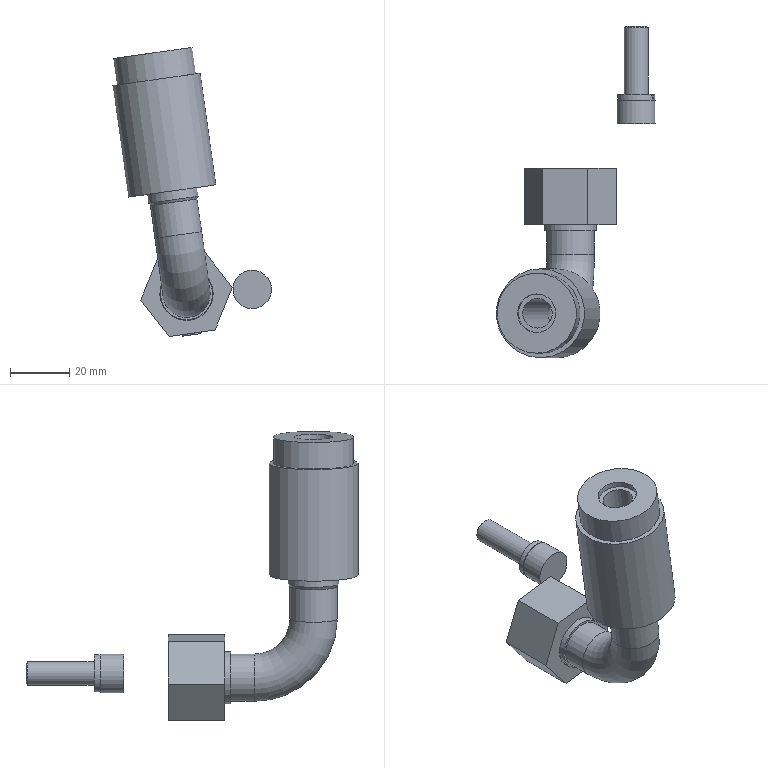Part | STEP file | COMPOUND | 6 solids | 135 faces | box 53.666 x 112 x 97.534 mm | volume 44207 mm3 | plane 73 | cylinder 29 | other 27 | cone 4 | torus 2 | commonest cylinder face diameters 13 x4 10 x2 16 x2 17 x2 27 x2 6.254 x1